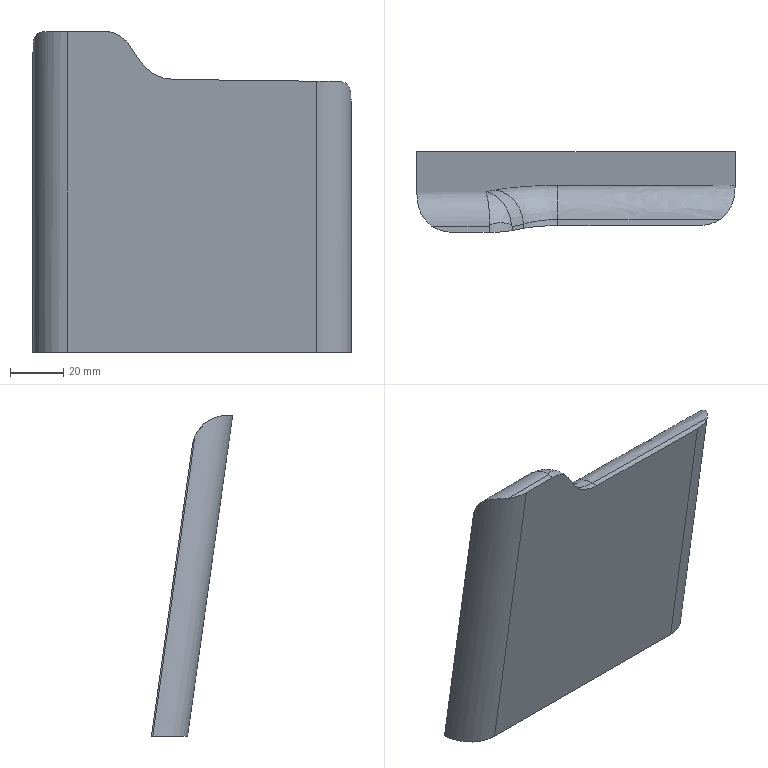Part | STEP file | solid 124 | 1 solid | 17 faces | box 120 x 30.646 x 121.053 mm | volume 166220 mm3 | spline 8 | plane 6 | cylinder 3 | commonest cylinder face diameters 26 x3